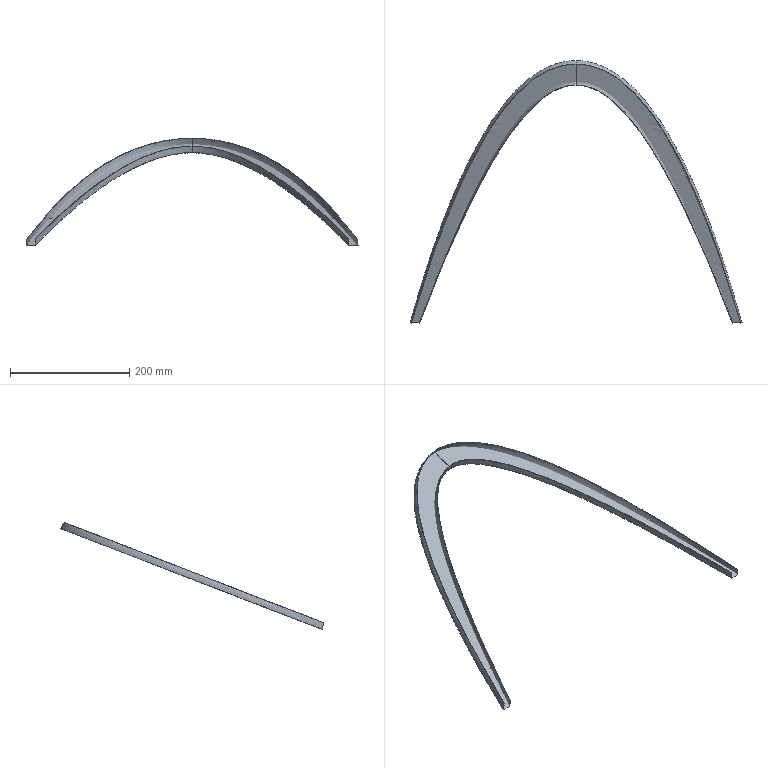Part | SolidWorks | features BaseBody 1 | 1 solid | 10 faces | box 556.796 x 440.276 x 180.135 mm | volume 233808 mm3 | spline 8 | plane 2